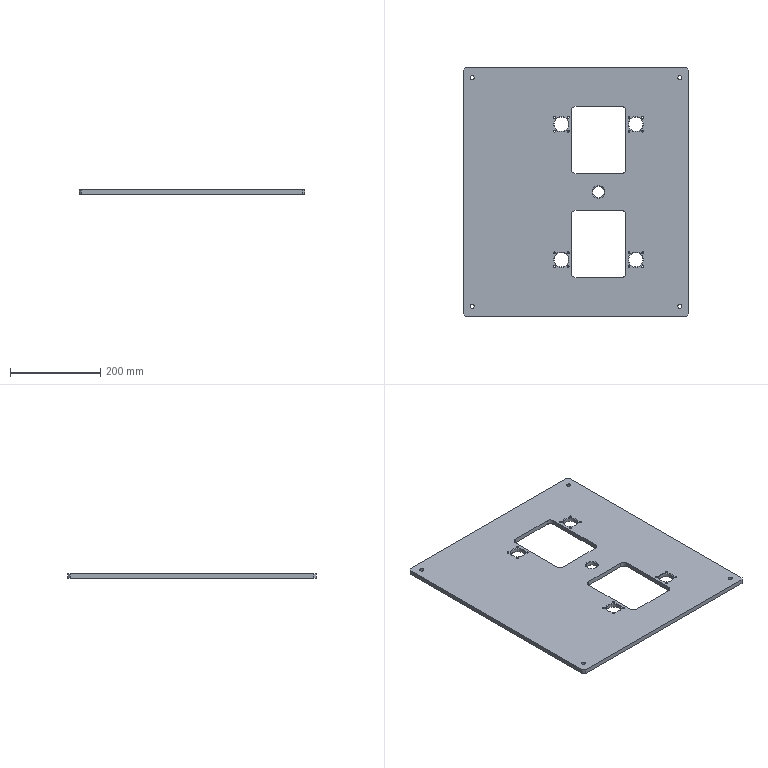CAM job | NX | 3-axis milling, drilling | part box 500 x 550 x 10 mm | stock box 504 x 554 x 10 mm
Tools:
number,name,description,diameter,corner_radius,flute_length,length,flutes
6,D8A45,Milling Tool-5 Parameters,8.0,0.0,50.0,75.0,2
13,4.2ZT,Drilling Tool,4.2,0.0,35.0,50.0,2
22,9.0ZT,Drilling Tool,9.0,0.0,35.0,50.0,2
4,D10,Milling Tool-5 Parameters,10.0,0.0,50.0,75.0,2
Operations:
program,operation,operation_type,tool,method,geometry_group,spindle_rpm,surface_speed,feed_per_tooth,feed_cut,feed_plunge,cut_length_mm,path_length_mm,cut_time_min,machine_time_min
1做里面,DRILLING,Operation,D8A45,METHOD,A,3500.0,65.0,0.0357,250.0,0.0,130.0,2330.889,0.52,0.7401
1做里面,DRILLING_1,Operation,4.2ZT,METHOD,A,2000.0,26.0,0.05,200.0,0.0,252.189,1594.883,1.261,1.395
1做里面,DRILLING_1_COPY,Operation,9.0ZT,METHOD,A,2000.0,26.0,0.05,200.0,0.0,68.816,1712.659,0.3441,0.5085
1做里面,HOLE_MILLING,CylinderMilling,D10,METHOD,A,7000.0,0.0,0.0,2000.0,100.0,5825.75,7298.131,2.913,3.06
1做里面,HOLE_MILLING_COPY,CylinderMilling,D10,METHOD,A,7000.0,0.0,0.0857,1200.0,100.0,1431.934,2851.816,1.193,1.335
1做里面,ADAPTIVE_MILLING,CavityMilling,D10,METHOD,A,7000.0,219.0,0.2143,3000.0,1000.0,50652.959,51100.695,17.878,17.922
1做里面,ZLEVEL_PROFILE_COPY,ZLevelMilling,D10,METHOD,A,7000.0,219.0,0.0714,1000.0,1000.0,993.65,1545.949,0.9936,1.049
1做里面,PLANAR_MILL_COPY,PlanarMilling,D8A45,METHOD,A,7000.0,1495.0,0.0893,1250.0,100.0,1856.713,7584.963,1.485,2.058
1做里面,PLANAR_MILL_COPY_COPY,PlanarMilling,D8A45,METHOD,A,7000.0,1495.0,0.0893,1250.0,100.0,507.334,1877.329,0.4059,0.5429
2做外面,ZLEVEL_PROFILE,ZLevelMilling,D10,METHOD,A,7000.0,219.0,0.2143,3000.0,1000.0,21309.922,21456.922,7.135,7.15
2做外面,ZLEVEL_PROFILE_COPY_COPY,ZLevelMilling,D10,METHOD,A,7000.0,219.0,0.0714,1000.0,1000.0,2125.039,2285.039,2.125,2.141
2做外面,PLANAR_MILL,PlanarMilling,D8A45,METHOD,A,7000.0,1495.0,0.0893,1250.0,100.0,2104.681,2244.681,1.684,1.698